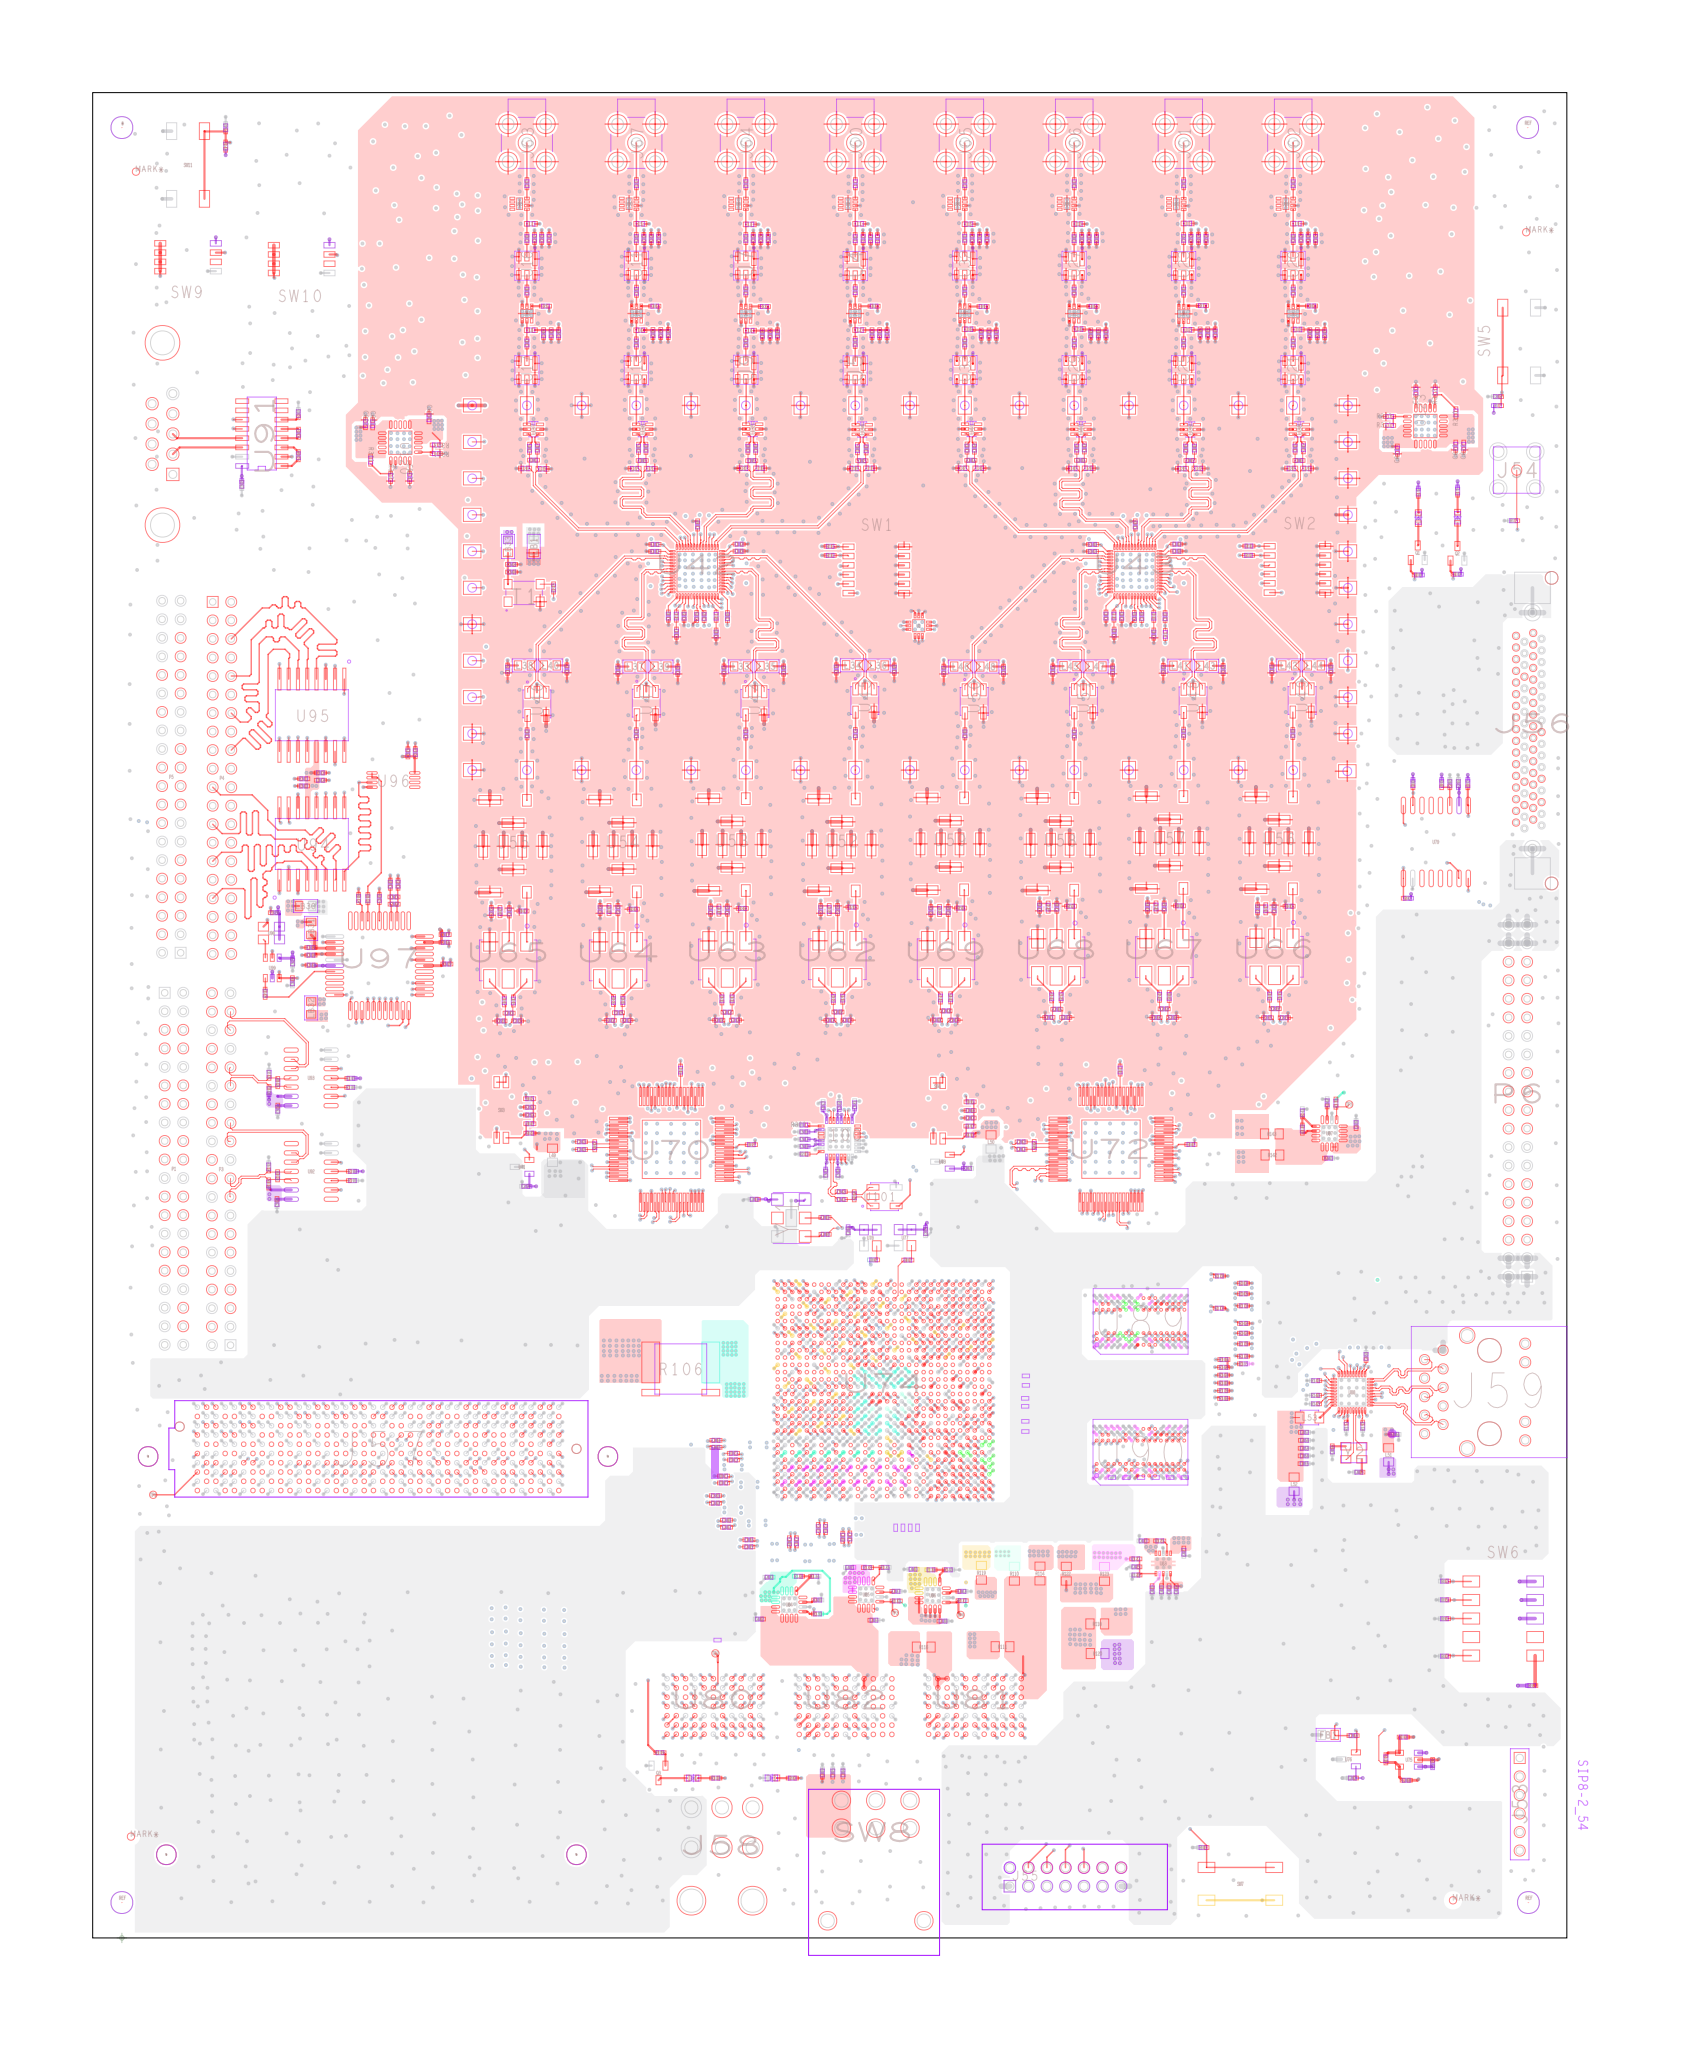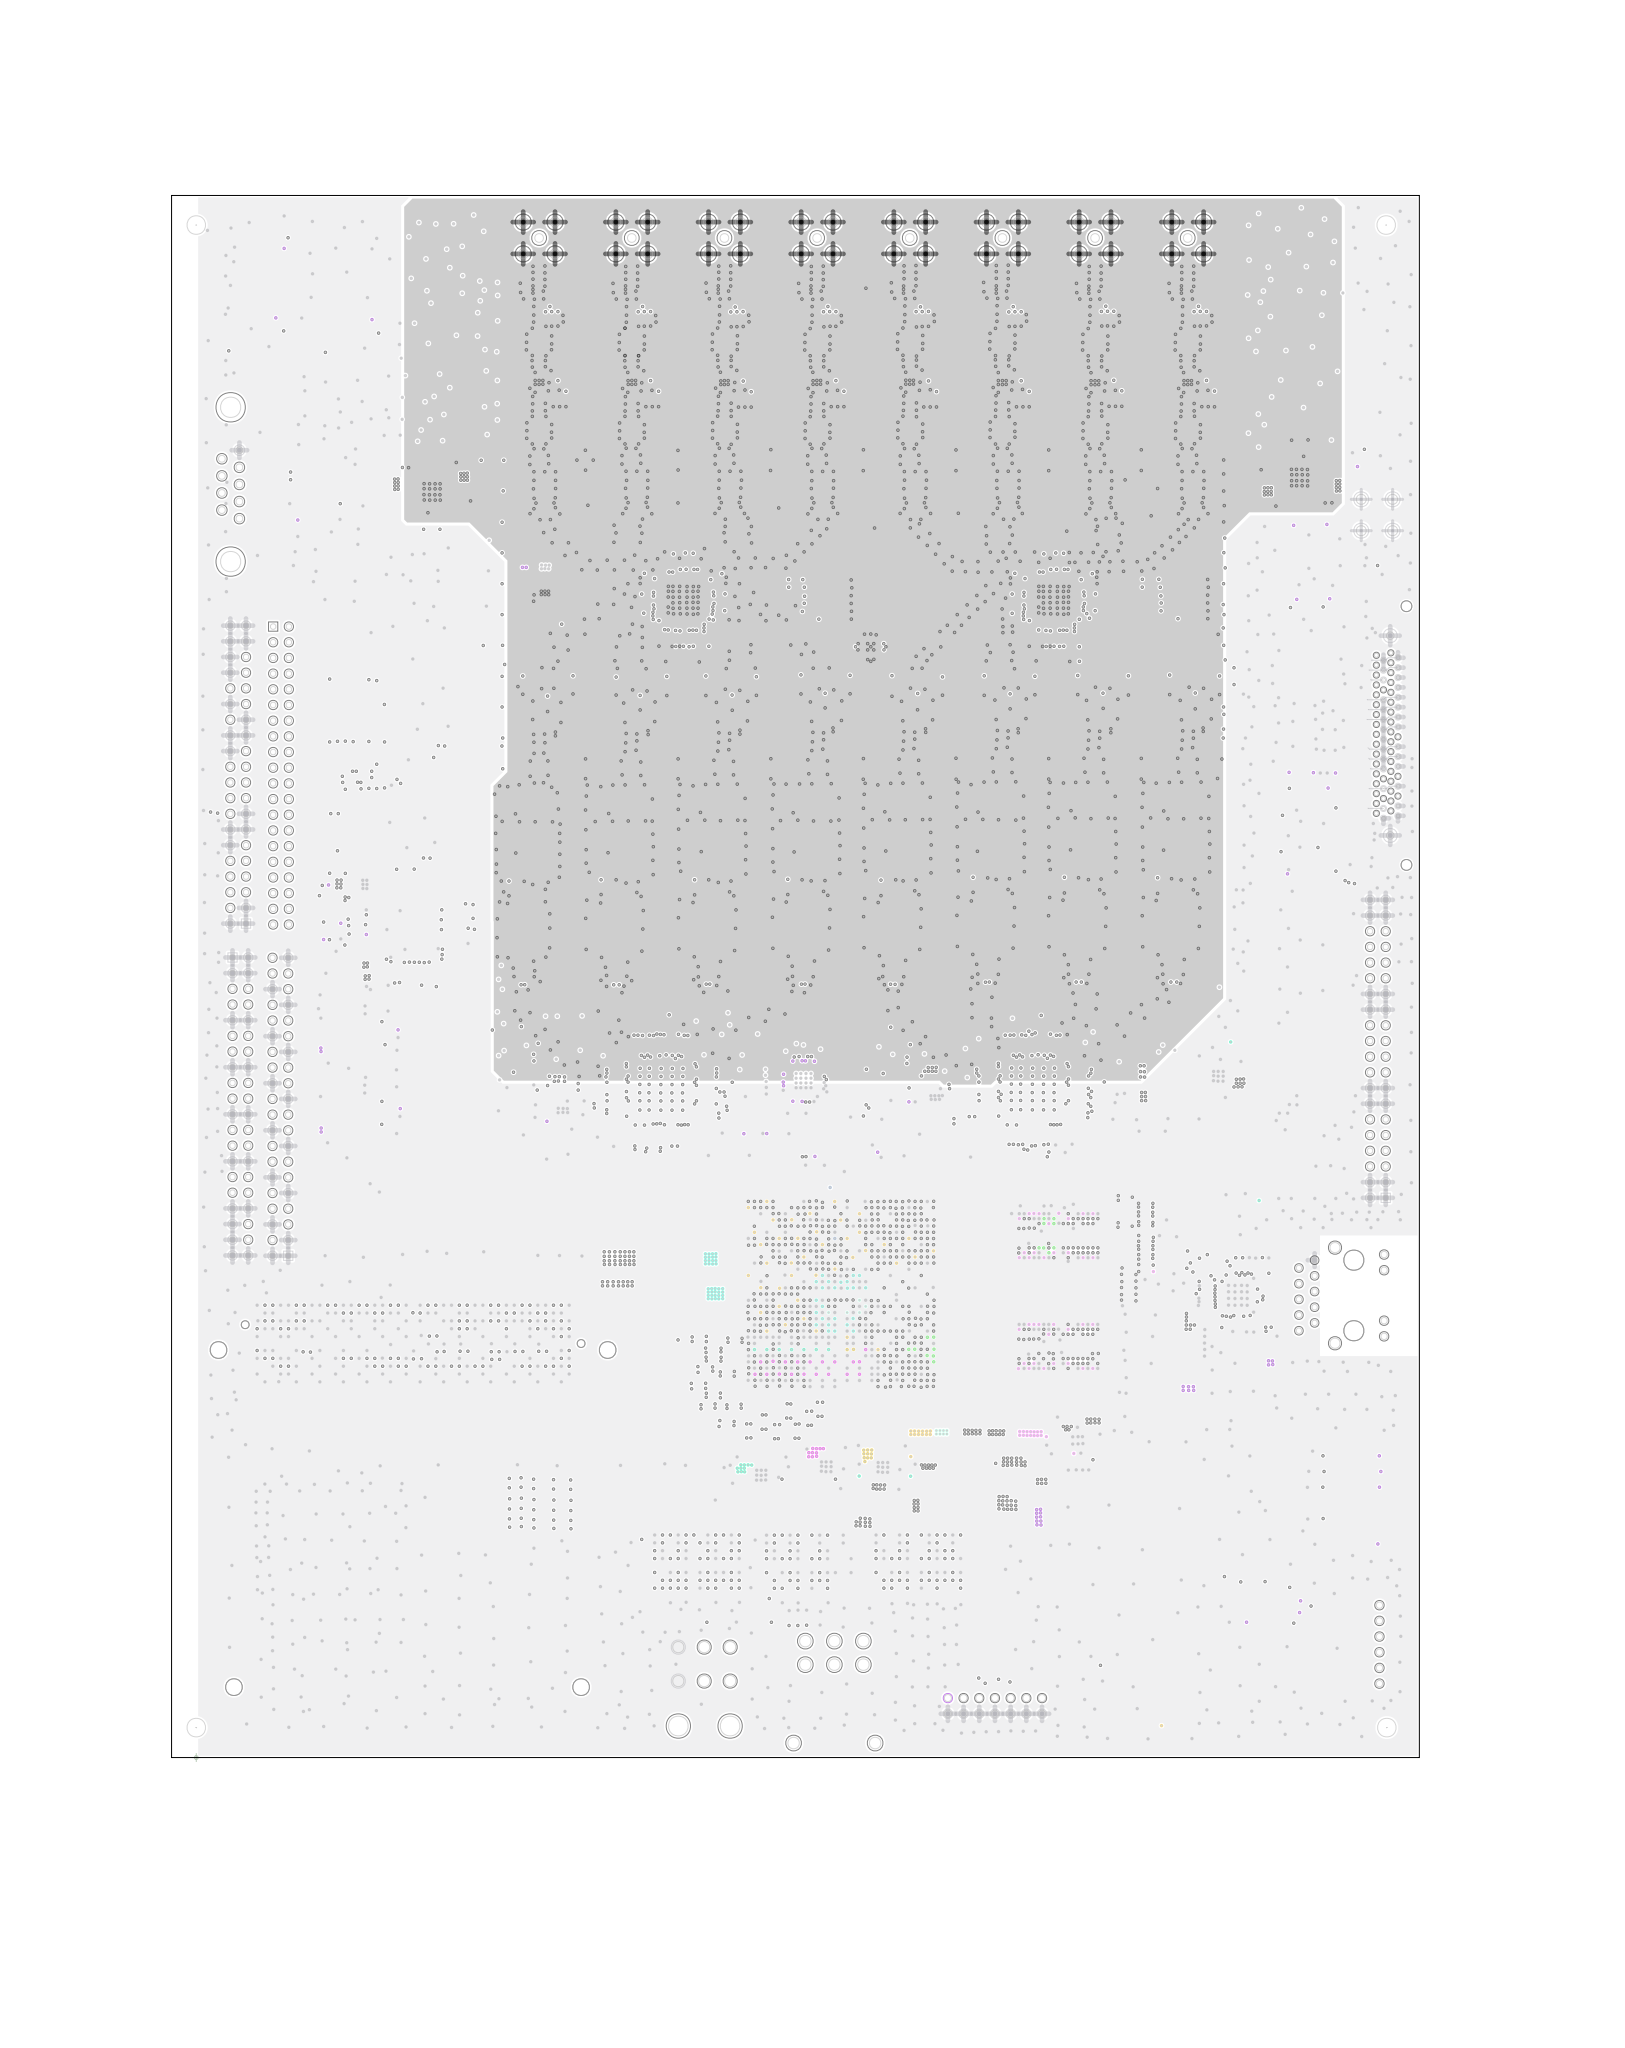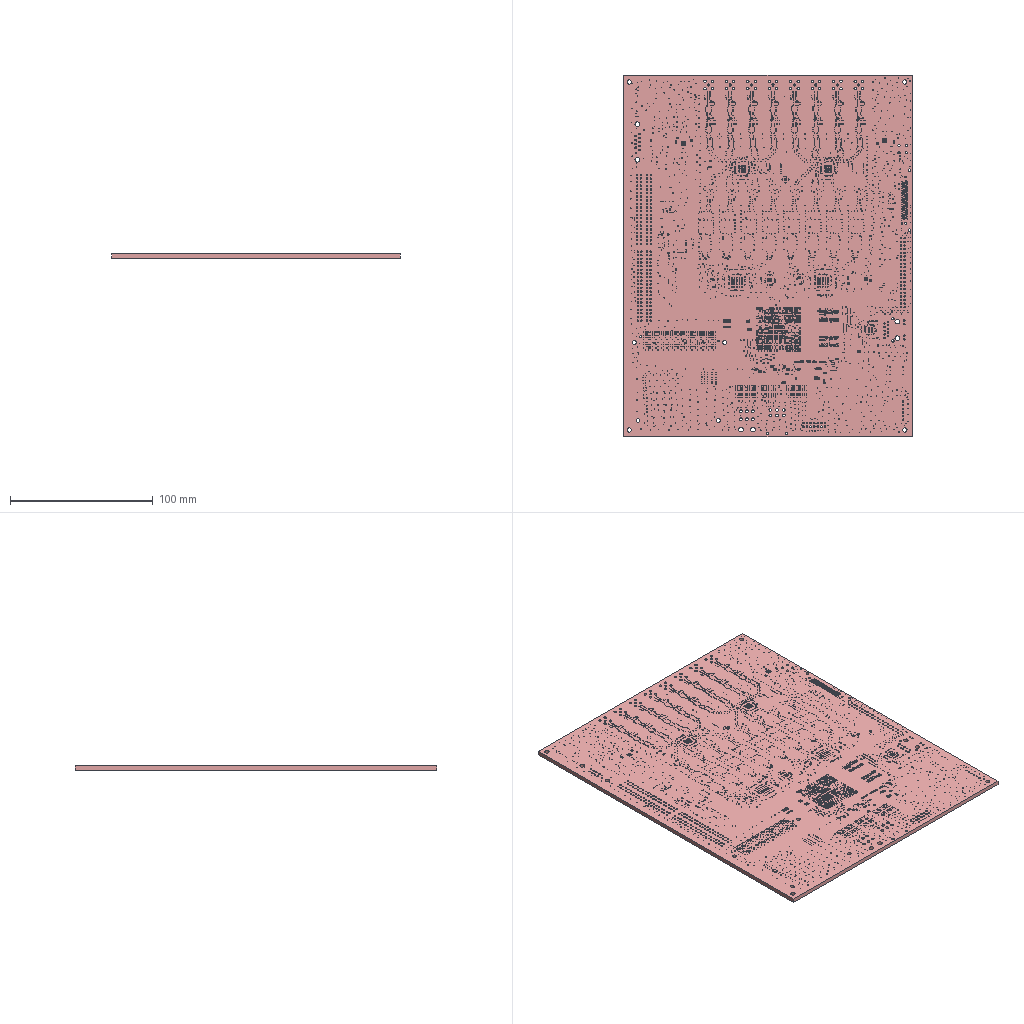Circuit board layout | Cadence Allegro | box 202 x 253 x 3 mm
Layer stack:
# Cadence Allegro layer stack of  (unit mm; from the constraint file cross-section; dielectric type: 0 not recorded (Allegro does not mark core vs prepreg), 3 surface material)
index,name,kind,layer,copper_thickness_mm,dielectric_type,dielectric_thickness_mm,dielectric_material,dielectric_constant
0,Top Surface,other,,,,,,
1,TOP,copper,TOP,0.0305,,,,
2,Dielectric1,dielectric,,,0,0.2032,FR-4,4.5
3,GND02,copper,GND02,0.0305,,,,
4,Dielectric2,dielectric,,,0,0.2032,FR-4,4.5
5,ART03,copper,ART03,0.0305,,,,
6,Dielectric3,dielectric,,,0,0.2032,FR-4,4.5
7,GND04,copper,GND04,0.0305,,,,
8,Dielectric4,dielectric,,,0,0.2032,FR-4,4.5
9,ART05,copper,ART05,0.0305,,,,
10,Dielectric5,dielectric,,,0,0.2032,FR-4,4.5
11,GND06,copper,GND06,0.0305,,,,
12,Dielectric6,dielectric,,,0,0.2032,FR-4,4.5
13,PWR07,copper,PWR07,0.0305,,,,
14,Dielectric7,dielectric,,,0,0.2032,FR-4,4.5
15,PWR08,copper,PWR08,0.0305,,,,
16,Dielectric8,dielectric,,,0,0.2032,FR-4,4.5
17,GND09,copper,GND09,0.0305,,,,
18,Dielectric9,dielectric,,,0,0.2032,FR-4,4.5
19,ART10,copper,ART10,0.0305,,,,
20,Dielectric10,dielectric,,,0,0.2032,FR-4,4.5
21,GND11,copper,GND11,0.0305,,,,
22,Dielectric11,dielectric,,,0,0.2032,FR-4,4.5
23,ART12,copper,ART12,0.0305,,,,
24,Dielectric12,dielectric,,,0,0.2032,FR-4,4.5
25,GND13,copper,GND13,0.0305,,,,
26,Dielectric13,dielectric,,,0,0.2032,FR-4,4.5
27,BOTTOM,copper,BOTTOM,0.0305,,,,
28,Bottom Surface,other,,,,,,
# drill layer pairs: low layer,high layer
drill_pair,TOP,BOTTOM
Part placement, first 520 of 1035 lines:
REFDES,COMP_VALUE,SYM_NAME,SYM_X,SYM_Y,SYM_ROTATE,SYM_MIRROR
C1,0.1uF,C0402,103.534,232.955,90.000,NO
C2,1000pF,C0402,101.578,232.98,90.000,NO
C3,10nF,C0402,102.594,232.955,90.000,NO
C4,0.1uF,C0402,104.851,219.939,90.000,NO
C5,1000pF,C0402,103.835,219.939,90.000,NO
C6,10nF,C0402,102.794,219.939,90.000,NO
C7,10nF,C0402,100.502,240.512,270.000,NO
C8,10nF,C0402,100.486,232.98,270.000,NO
C9,10nF,C0402,100.486,225.843,270.000,NO
C10,10nF,C0402,100.486,218.756,270.000,NO
C11,0.1uF,C0402,88.57,232.994,90.000,NO
C12,1000pF,C0402,86.512,232.994,90.000,NO
C13,10nF,C0402,87.554,232.994,90.000,NO
C14,0.1uF,C0402,89.84,219.913,90.000,NO
C15,1000pF,C0402,88.824,219.888,90.000,NO
C16,10nF,C0402,87.757,219.888,90.000,NO
C17,10nF,C0402,85.503,240.512,270.000,NO
C18,10nF,C0402,85.5,233.006,270.000,NO
C19,10nF,C0402,85.5,225.818,270.000,NO
C20,10nF,C0402,85.5,218.68,270.000,NO
C21,0.1uF,C0402,73.558,232.994,90.000,NO
C22,1000pF,C0402,71.526,232.994,90.000,NO
C23,10nF,C0402,72.542,232.994,90.000,NO
C24,0.1uF,C0402,72.771,219.964,90.000,NO
C25,1000pF,C0402,73.838,219.964,90.000,NO
C26,10nF,C0402,74.879,219.964,90.000,NO
C27,10nF,C0402,70.502,240.512,270.000,NO
C28,10nF,C0402,70.488,233.006,270.000,NO
C29,10nF,C0402,70.514,225.767,270.000,NO
C30,10nF,C0402,70.488,218.68,270.000,NO
C31,0.1uF,C0402,58.547,233.02,90.000,NO
C32,1000pF,C0402,56.54,233.02,90.000,NO
C33,10nF,C0402,57.531,233.02,90.000,NO
C34,0.1uF,C0402,57.785,219.939,90.000,NO
C35,1000pF,C0402,58.826,219.939,90.000,NO
C36,10nF,C0402,59.842,219.939,90.000,NO
C37,10nF,C0402,55.502,240.512,270.000,NO
C38,10nF,C0402,55.502,233.004,270.000,NO
C39,10nF,C0402,55.502,225.792,270.000,NO
C40,10nF,C0402,55.502,218.68,270.000,NO
C41,0.1uF,C0402,163.576,233.02,90.000,NO
C42,1000pF,C0402,161.569,233.02,90.000,NO
C43,10nF,C0402,162.56,233.045,90.000,NO
C44,0.1uF,C0402,164.821,219.939,90.000,NO
C45,1000pF,C0402,163.805,219.939,90.000,NO
C46,10nF,C0402,162.789,219.939,90.000,NO
C47,10nF,C0402,160.502,240.512,270.000,NO
C48,10nF,C0402,160.506,233.006,270.000,NO
C49,10nF,C0402,160.506,225.792,270.000,NO
C50,10nF,C0402,160.506,218.68,270.000,NO
C51,0.1uF,C0402,148.565,233.02,90.000,NO
C52,1000pF,C0402,146.482,233.02,90.000,NO
C53,10nF,C0402,147.523,233.02,90.000,NO
C54,0.1uF,C0402,149.809,220.04,90.000,NO
C55,1000pF,C0402,148.793,220.04,90.000,NO
C56,10nF,C0402,147.752,220.04,90.000,NO
C57,10nF,C0402,145.502,240.512,270.000,NO
C58,10nF,C0402,145.494,233.006,270.000,NO
C59,10nF,C0402,145.494,225.792,270.000,NO
C60,10nF,C0402,145.494,218.68,270.000,NO
C61,0.1uF,C0402,133.553,232.969,90.000,NO
C62,1000pF,C0402,131.521,232.994,90.000,NO
C63,10nF,C0402,132.537,232.969,90.000,NO
C64,0.1uF,C0402,134.849,219.913,90.000,NO
C65,1000pF,C0402,133.807,219.913,90.000,NO
C66,10nF,C0402,132.766,219.913,90.000,NO
C67,10nF,C0402,130.502,240.512,270.000,NO
C68,10nF,C0402,130.483,232.98,270.000,NO
C69,10nF,C0402,130.483,225.792,270.000,NO
C70,10nF,C0402,130.508,218.68,270.000,NO
C71,0.1uF,C0402,118.542,233.045,90.000,NO
C72,1000pF,C0402,116.51,233.02,90.000,NO
C73,10nF,C0402,117.526,233.02,90.000,NO
C74,0.1uF,C0402,119.812,219.888,90.000,NO
C75,1000pF,C0402,118.821,219.888,90.000,NO
C76,10nF,C0402,117.754,219.888,90.000,NO
C77,10nF,C0402,115.502,240.512,270.000,NO
C78,10nF,C0402,115.497,233.031,270.000,NO
C79,10nF,C0402,115.497,225.792,270.000,NO
C80,10nF,C0402,115.497,218.68,270.000,NO
C81,39pF,C0402,100.794,204.186,270.000,NO
C82,NC,C0402,101.404,202.535,180.000,NO
C83,39pF,C0402,101.988,204.161,270.000,NO
C84,39pF,C0402,85.783,204.237,270.000,NO
C85,NC,C0402,86.309,202.54,180.000,NO
C86,39pF,C0402,86.85,204.237,270.000,NO
C87,39pF,C0402,70.797,204.237,270.000,NO
C88,NC,C0402,71.305,202.56,180.000,NO
C89,39pF,C0402,71.813,204.237,270.000,NO
C90,39pF,C0402,55.861,204.237,270.000,NO
C91,NC,C0402,56.395,202.611,180.000,NO
C92,39pF,C0402,56.928,204.262,270.000,NO
C93,39pF,C0402,160.763,204.262,270.000,NO
C94,NC,C0402,161.297,202.56,180.000,NO
C95,39pF,C0402,161.906,204.313,270.000,NO
C96,39pF,C0402,145.777,204.262,270.000,NO
C97,NC,C0402,146.362,202.56,180.000,NO
C98,39pF,C0402,146.971,204.262,270.000,NO
C99,39pF,C0402,130.842,204.262,270.000,NO
C100,NC,C0402,131.369,202.59,180.000,NO
C101,39pF,C0402,131.883,204.288,270.000,NO
C102,39pF,C0402,115.805,204.262,270.000,NO
C103,NC,C0402,116.332,202.59,180.000,NO
C104,39pF,C0402,116.822,204.262,270.000,NO
C105,10nF,C0402,79.781,181.178,90.000,NO
C106,10nF,C0402,82.982,181.153,270.000,NO
C107,NC,C0402,75.997,178.892,270.000,NO
C108,NC,C0402,76.403,183.82,270.000,YES
C109,NC,C0402,81.432,178.765,270.000,NO
C110,NC,C0402,81.458,183.845,270.000,YES
C111,1uF,C0402,79.451,190.805,270.000,YES
C112,1uF,C0402,84.582,191.094,180.000,NO
C113,1uF,C0402,80.467,190.805,270.000,YES
C114,1uF,C0402,77.165,190.83,270.000,YES
C115,1uF,C0402,73.05,191.059,0.000,NO
C116,1uF,C0402,82.398,188.9,180.000,YES
C117,1uF,C0402,82.372,187.935,180.000,YES
C118,1uF,C0402,75.26,187.96,0.000,YES
C119,1uF,C0402,75.26,188.9,0.000,YES
C120,1uF,C0402,75.235,185.395,0.000,YES
C121,1uF,C0402,77.419,183.845,90.000,YES
C122,1uF,C0402,78.435,183.845,90.000,YES
C123,1uF,C0402,82.372,185.953,180.000,YES
C124,1uF,C0402,79.451,183.845,90.000,YES
C125,1uF,C0402,84.582,190.128,0.000,NO
C126,1uF,C0402,82.398,186.969,0.000,YES
C127,1uF,C0402,80.467,183.845,270.000,YES
C128,1uF,C0402,78.765,181.178,270.000,NO
C129,1uF,C0402,77.038,181.204,270.000,NO
C130,1uF,C0402,74.879,181.229,270.000,NO
C131,1uF,C0402,75.235,186.334,180.000,YES
C132,1uF,C0402,73.025,190.094,180.000,NO
C133,1uF,C0402,76.175,190.83,90.000,YES
C134,33nF,C0402,78.892,193.726,90.000,NO
C135,1uF,C0402,81.432,190.83,90.000,YES
C136,10nF,C0402,139.751,181.178,90.000,NO
C137,10nF,C0402,142.951,181.153,270.000,NO
C138,NC,C0402,135.966,178.892,270.000,NO
C139,NC,C0402,136.373,183.82,270.000,YES
C140,NC,C0402,141.402,178.765,270.000,NO
C141,NC,C0402,141.427,183.845,270.000,YES
C142,1uF,C0402,139.421,190.822,270.000,YES
C143,1uF,C0402,144.552,191.094,180.000,NO
C144,1uF,C0402,140.437,190.805,270.000,YES
C145,1uF,C0402,137.135,190.83,270.000,YES
C146,1uF,C0402,133.02,191.059,0.000,NO
C147,1uF,C0402,142.367,188.9,180.000,YES
C148,1uF,C0402,142.342,187.935,180.000,YES
C149,1uF,C0402,135.23,187.96,0.000,YES
C150,1uF,C0402,135.23,188.9,0.000,YES
C151,1uF,C0402,135.204,185.395,0.000,YES
C152,1uF,C0402,137.389,183.845,90.000,YES
C153,1uF,C0402,138.405,183.845,90.000,YES
C154,1uF,C0402,142.342,185.953,180.000,YES
C155,1uF,C0402,139.421,183.845,90.000,YES
C156,1uF,C0402,144.552,190.128,0.000,NO
C157,1uF,C0402,142.367,186.969,0.000,YES
C158,1uF,C0402,140.437,183.845,270.000,YES
C159,1uF,C0402,138.735,181.178,270.000,NO
C160,1uF,C0402,137.008,181.204,270.000,NO
C161,1uF,C0402,134.849,181.229,270.000,NO
C162,1uF,C0402,135.204,186.334,180.000,YES
C163,1uF,C0402,132.994,190.094,180.000,NO
C164,1uF,C0402,136.144,190.852,90.000,YES
C165,33nF,C0402,138.862,193.726,90.000,NO
C166,1uF,C0402,141.402,190.83,90.000,YES
C167,0.1uF,C0402,82.499,173.83,270.000,NO
C168,0.1uF,C0402,105.842,173.957,270.000,NO
C169,0.1uF,C0402,90.678,173.83,270.000,NO
C170,0.1uF,C0402,97.892,173.982,270.000,NO
C171,1nF,C0402,101.803,171.247,270.000,YES
C172,1nF,C0402,86.766,170.84,270.000,YES
C173,10nF,C0402,100.508,165.116,270.000,NO
C174,10nF,C0402,85.496,165.065,270.000,NO
C175,0.1uF,C0402,52.857,173.957,270.000,NO
C176,0.1uF,C0402,76.175,173.804,270.000,NO
C177,0.1uF,C0402,60.985,173.982,270.000,NO
C178,0.1uF,C0402,67.97,173.83,270.000,NO
C179,1nF,C0402,71.857,170.891,270.000,YES
C180,1nF,C0402,56.871,170.79,270.000,YES
C181,10nF,C0402,70.485,165.091,270.000,NO
C182,10nF,C0402,55.524,165.091,270.000,NO
C183,0.1uF,C0402,150.901,173.906,270.000,NO
C184,0.1uF,C0402,157.582,173.957,270.000,NO
C185,0.1uF,C0402,142.697,173.906,270.000,NO
C186,0.1uF,C0402,165.659,173.957,270.000,NO
C187,1nF,C0402,161.722,171.247,270.000,YES
C188,1nF,C0402,146.812,171.196,270.000,YES
C189,10nF,C0402,160.452,165.141,270.000,NO
C190,10nF,C0402,145.491,165.167,270.000,NO
C191,0.1uF,C0402,127.559,173.83,270.000,NO
C192,0.1uF,C0402,112.624,173.804,270.000,NO
C193,0.1uF,C0402,135.763,173.83,270.000,NO
C194,0.1uF,C0402,120.802,173.804,270.000,NO
C195,1nF,C0402,131.75,171.12,270.000,YES
C196,1nF,C0402,116.764,171.12,270.000,YES
C197,10nF,C0402,130.505,165.065,270.000,NO
C198,10nF,C0402,115.519,165.091,270.000,NO
C207,5pF,C0402,99.365,125.832,180.000,NO
C208,5pF,C0402,98.12,126.949,0.000,NO
C209,0.1uF,C0402,98.069,140.995,270.000,NO
C210,0.1uF,C0402,95.758,140.995,90.000,NO
C211,5pF,C0402,97.028,125.822,0.000,NO
C212,5pF,C0402,84.074,125.832,180.000,NO
C213,5pF,C0402,82.931,126.924,0.000,NO
C214,0.1uF,C0402,82.956,140.919,270.000,NO
C215,0.1uF,C0402,80.67,140.919,90.000,NO
C216,5pF,C0402,81.788,125.822,0.000,NO
C217,5pF,C0402,69.19,125.806,180.000,NO
C218,5pF,C0402,68.047,126.848,0.000,NO
C219,0.1uF,C0402,67.97,140.986,270.000,NO
C220,0.1uF,C0402,65.532,140.986,90.000,NO
C221,5pF,C0402,66.929,125.806,0.000,NO
C222,5pF,C0402,54.204,125.73,180.000,NO
C223,5pF,C0402,53.061,126.797,0.000,NO
C224,0.1uF,C0402,53.086,140.681,270.000,NO
C225,0.1uF,C0402,50.622,140.716,90.000,NO
C226,5pF,C0402,51.943,125.721,0.000,NO
C227,5pF,C0402,159.283,126.162,180.000,NO
C228,5pF,C0402,158.039,127.406,0.000,NO
C229,0.1uF,C0402,157.886,141.097,270.000,NO
C230,0.1uF,C0402,155.626,141.097,90.000,NO
C231,5pF,C0402,156.972,126.162,0.000,NO
C232,5pF,C0402,143.993,126.213,180.000,NO
C233,5pF,C0402,142.824,127.381,0.000,NO
C234,0.1uF,C0402,142.824,141.351,270.000,NO
C235,0.1uF,C0402,140.538,141.351,90.000,NO
C236,5pF,C0402,141.707,126.187,0.000,NO
C237,5pF,C0402,129.337,126.213,180.000,NO
C238,5pF,C0402,128.118,127.33,0.000,NO
C239,0.1uF,C0402,128.118,141.326,270.000,NO
C240,0.1uF,C0402,125.755,141.326,90.000,NO
C241,5pF,C0402,127.025,126.213,0.000,NO
C242,5pF,C0402,114.021,125.832,180.000,NO
C243,5pF,C0402,112.928,127.102,0.000,NO
C244,0.1uF,C0402,113.233,140.868,270.000,NO
C245,0.1uF,C0402,110.846,140.843,90.000,NO
C246,5pF,C0402,111.633,125.848,0.000,NO
C247,0.1uF,C0402,62.966,109.16,180.000,NO
C248,0.1uF,C0402,62.966,108.093,180.000,NO
C249,10uF,C0402,75.032,115.621,270.000,YES
C250,10uF,C0402,55.347,103.048,0.000,NO
C251,1.0uF,C0402,55.88,113.894,180.000,NO
C252,0.1uF,C0402,55.88,112.827,0.000,NO
C253,0.1uF,C0402,67.869,106.35,0.000,YES
C254,0.1uF,C0402,82.779,105.867,180.000,YES
C255,0.1uF,C0402,67.843,107.391,0.000,YES
C256,0.1uF,C0402,78.054,115.621,270.000,YES
C257,0.1uF,C0402,82.956,110.388,180.000,YES
C258,0.1uF,C0402,73.533,115.621,270.000,YES
C259,0.1uF,C0402,67.843,110.338,0.000,YES
C260,0.1uF,C0402,72.06,115.57,270.000,YES
C261,0.1uF,C0402,67.843,109.347,0.000,YES
C262,0.1uF,C0402,123.231,109.144,180.000,NO
C263,0.1uF,C0402,123.199,108.128,180.000,NO
C264,10uF,C0402,135.28,115.621,270.000,YES
C265,10uF,C0402,115.875,105.512,180.000,NO
C266,1.0uF,C0402,116.23,113.436,180.000,NO
C267,0.1uF,C0402,116.23,112.42,0.000,NO
C268,0.1uF,C0402,128.092,106.375,0.000,YES
C269,0.1uF,C0402,143.002,105.893,180.000,YES
C270,0.1uF,C0402,128.067,109.372,0.000,YES
C271,0.1uF,C0402,128.067,107.417,0.000,YES
C272,0.1uF,C0402,138.278,115.646,270.000,YES
C273,0.1uF,C0402,132.283,115.595,270.000,YES
C274,0.1uF,C0402,143.213,110.414,180.000,YES
C275,0.1uF,C0402,133.756,115.646,270.000,YES
C276,0.1uF,C0402,128.067,110.363,0.000,YES
C277,0.1uF/25V/X2R,C0402_BGA,103.327,73.584,180.000,YES
C278,0.1uF/25V/X2R,C0402_BGA,104.851,73.05,90.000,YES
C279,10uF,C0402,179.603,23.901,270.000,NO
C280,10uF,C0402,175.997,21.615,180.000,NO
C281,47uF/10V/X5R,C0402_BGA,104.877,69.063,90.000,YES
C282,10uF,C0402,168.605,21.92,0.000,NO
C283,10uF/10V,C0402,188.493,211.328,0.000,NO
C284,10uF,C0402,168.707,27.737,0.000,NO
C285,0.1uF,C0402,110.134,96.85,90.000,NO
C286,0.1uF,C0402,99.517,96.952,90.000,NO
C287,100uF/6.3V/X5R,C0402_BGA,100.355,83.566,180.000,YES
C288,100uF/6.3V/X5R,C0402_BGA,105.893,85.065,90.000,YES
C289,0.1uF,C0402,96.342,98.781,180.000,NO
C290,0.1uF,C0402,96.368,96.469,180.000,NO
C291,0.1uF,C0402,86.639,101.27,0.000,NO
C292,0.1uF,C0402,183.134,158.267,270.000,NO
C293,0.1uF,C0402,181.966,158.267,270.000,NO
C294,0.1uF/25V/X7R,C0402_BGA,114.351,73.609,0.000,YES
C295,0.1uF/25V/X7R,C0402_BGA,114.351,72.568,0.000,YES
C296,0.1uF/25V/X7R,C0402_BGA,116.357,76.581,180.000,YES
C297,0.1uF/25V/X7R,C0402_BGA,111.887,71.095,90.000,YES
C298,100uF/6.3V/X5R,C0402_BGA,114.351,69.571,0.000,YES
C299,100uF/6.3V/X5R,C0402_BGA,113.386,77.572,180.000,YES
C300,0.1uF/25V/X7R,C0402_BGA,113.386,66.599,0.000,YES
C301,0.1uF/25V/X7R,C0402_BGA,115.341,67.589,0.000,YES
C302,100uF/6.3V/X5R,C0402_BGA,112.852,61.112,270.000,YES
C303,100uF/6.3V/X5R,C0402_BGA,111.379,88.57,0.000,YES
C304,0.1uF,C0402,81.407,68.224,0.000,NO
C305,0.1uF,C0402,81.407,67.259,0.000,NO
C306,0.1uF,C0402,82.448,63.322,0.000,NO
C307,0.1uF,C0402,85.979,62.611,180.000,YES
C308,0.1uF,C0402,85.954,61.62,180.000,YES
C309,0.1uF,C0402,91.465,54.305,90.000,NO
C310,0.1uF,C0402,82.448,62.382,0.000,NO
C311,0.1uF,C0402,92.431,54.305,90.000,NO
C312,0.1uF,C0402,83.795,65.532,0.000,NO
C313,0.1uF,C0402,87.224,67.056,180.000,YES
C314,0.1uF,C0402,83.795,66.446,0.000,NO
C315,0.1uF,C0402,87.224,68.021,180.000,YES
C316,0.1uF,C0402,83.769,64.999,180.000,YES
C317,0.1uF,C0402,95.428,56.134,90.000,NO
C318,0.1uF,C0402,83.769,64.084,180.000,YES
C319,0.1uF,C0402,96.418,56.134,90.000,NO
C320,0.1uF,C0402,87.071,57.302,180.000,YES
C321,0.1uF,C0402,101.473,56.413,270.000,YES
C322,0.1uF,C0402,87.071,56.388,180.000,YES
C323,0.1uF,C0402,100.508,56.413,270.000,YES
C324,0.1uF,C0402,96.774,52.857,90.000,YES
C325,0.1uF,C0402,97.714,52.857,90.000,YES
C326,0.1uF,C0402,98.781,54.94,270.000,NO
C327,0.1uF,C0402,99.746,54.966,270.000,NO
C328,0.1uF,C0402,93.497,52.781,90.000,YES
C329,0.1uF,C0402,94.437,52.781,90.000,YES
C330,0.1uF,C0402,88.951,52.908,90.000,YES
C331,0.1uF,C0402,89.941,52.908,90.000,YES
C332,0.1uF,C0402,81.331,60.63,0.000,NO
C333,0.1uF,C0402,81.331,59.614,0.000,NO
C334,0.1uF,C0402,85.928,54.585,180.000,NO
C335,0.1uF,C0402,85.903,53.619,180.000,NO
C336,0.1uF,C0402,82.855,57.277,0.000,NO
C337,0.1uF,C0402,82.855,56.312,0.000,NO
C338,0.1uF,C0402,83.718,59.131,0.000,YES
C339,0.1uF,C0402,83.718,58.166,0.000,YES
C340,100uF/6.3V/X5R,C0402_BGA,116.357,83.566,0.000,YES
C341,100uF/6.3V/X5R,C0402_BGA,106.883,82.042,90.000,YES
C342,100uF/6.3V/X5R,C0402_BGA,94.869,83.083,270.000,YES
C343,100uF/6.3V/X5R,C0402_BGA,93.853,72.06,270.000,YES
C344,4.7uF/6.3V/X5R,C0402_BGA,102.362,74.803,180.000,YES
C345,4.7uF/6.3V/X5R,C0402_BGA,102.358,76.574,180.000,YES
C346,4.7uF/6.3V/X5R,C0402_BGA,104.419,75.667,180.000,YES
C347,4.7uF/6.3V/X5R,C0402_BGA,104.419,76.556,180.000,YES
C348,4.7uF/6.3V/X5R,C0402_BGA,108.407,76.556,0.000,YES
C349,4.7uF/6.3V/X5R,C0402_BGA,100.355,74.803,180.000,YES
C350,4.7uF/6.3V/X5R,C0402_BGA,100.358,76.574,180.000,YES
C351,4.7uF/6.3V/X5R,C0402_BGA,100.355,75.641,180.000,YES
C352,4.7uF/6.3V/X5R,C0402_BGA,108.407,75.616,0.000,YES
C353,330uF/10V/TANT,C0402_BGA,102.362,75.667,0.000,YES
C354,330uF/10V/TANT,C0402_BGA,102.387,69.596,0.000,YES
C355,330uF/10V/TANT,C0402_BGA,107.366,77.572,180.000,YES
C356,330uF/10V/TANT,C0402_BGA,101.346,71.603,180.000,YES
C357,330uF/10V/TANT,C0402_BGA,106.858,72.085,270.000,YES
C358,330uF/10V/TANT,C0402_BGA,101.371,77.572,0.000,YES
C359,47uF/10V/X5R,C0402_BGA,102.362,72.517,0.000,YES
C360,47uF/10V/X5R,C0402_BGA,107.899,72.06,270.000,YES
C361,47uF/10V/X5R,C0402_BGA,108.204,74.574,0.000,YES
C362,47uF/10V/X5R,C0402_BGA,107.899,70.053,90.000,YES
C363,0.022uF/10V/X5R,C0402_BGA,99.873,61.062,270.000,YES
C364,0.022uF/10V/X5R,C0402_BGA,97.892,61.087,270.000,YES
C365,0.022uF/10V/X5R,C0402_BGA,95.91,61.062,270.000,YES
C366,0.022uF/10V/X5R,C0402_BGA,102.87,64.084,90.000,YES
C367,0.022uF/10V/X5R,C0402_BGA,93.929,66.091,90.000,YES
C368,0.022uF/10V/X5R,C0402_BGA,100.813,66.091,90.000,YES
C369,0.022uF/10V/X5R,C0402_BGA,91.948,65.1,270.000,YES
C370,0.022uF/10V/X5R,C0402_BGA,101.879,66.091,90.000,YES
C371,0.022uF/10V/X5R,C0402_BGA,105.893,65.024,270.000,YES
C372,0.022uF/10V/X5R,C0402_BGA,104.927,65.049,270.000,YES
C373,0.022uF/10V/X5R,C0402_BGA,104.927,67.081,90.000,YES
C374,0.022uF/10V/X5R,C0402_BGA,105.893,67.031,90.000,YES
C375,0.47uF/10V/X5R,C0402_BGA,93.929,61.062,270.000,YES
C376,0.47uF/10V/X5R,C0402_BGA,101.93,61.036,270.000,YES
C377,0.47uF/10V/X5R,C0402_BGA,107.874,61.087,270.000,YES
C378,0.47uF/10V/X5R,C0402_BGA,107.874,63.094,270.000,YES
C379,0.47uF/10V/X5R,C0402_BGA,89.865,66.116,90.000,YES
C380,0.47uF/10V/X5R,C0402_BGA,95.91,66.091,90.000,YES
C381,0.47uF/10V/X5R,C0402_BGA,96.85,66.091,90.000,YES
C382,0.47uF/10V/X5R,C0402_BGA,98.831,65.101,270.000,YES
C383,1uF/25V/X5R,C0402_BGA,91.872,61.062,270.000,YES
C384,1uF/25V/X5R,C0402_BGA,89.916,61.138,270.000,YES
C385,4.7uF/6.3V/X5R,C0402_BGA,105.842,61.062,270.000,YES
C386,4.7uF/6.3V/X5R,C0402_BGA,108.839,65.024,270.000,YES
C387,1uF/25V/X5R,C0402_BGA,92.888,65.1,270.000,YES
C388,1uF/25V/X5R,C0402_BGA,97.917,65.1,270.000,YES
C389,4.7uF/6.3V/X5R,C0402_BGA,91.008,66.116,90.000,YES
C390,4.7uF/6.3V/X5R,C0402_BGA,94.996,66.091,90.000,YES
C391,47uF,C0402,78.664,35.433,0.000,YES
C392,47uF,C0402,74.854,35.484,0.000,YES
C393,47uF,C0402,83.439,35.433,0.000,YES
C394,47uF,C0402,98.806,22.631,270.000,NO
C395,10uF,C0402,97.409,22.622,270.000,NO
C396,10uF,C0402,87.224,31.648,0.000,YES
C397,47uF,C0402,87.249,35.458,0.000,YES
C398,100uF/16V,C0402,83.439,31.623,180.000,YES
C399,10uF,C0402,95.986,22.622,270.000,NO
C400,0.1uF,C0402,79.858,29.464,90.000,YES
C401,10uF,C0402,78.613,31.648,0.000,YES
C402,4.7uF,C0402,77.572,29.337,180.000,YES
C403,10uF,C0402,74.778,31.674,0.000,YES
C404,10uF,C0402,123.038,31.674,0.000,YES
C405,10uF,C0402,119.202,31.648,0.000,YES
C406,47uF,C0402,123.012,35.433,0.000,YES
C407,0.1uF,C0402,124.384,29.388,90.000,YES
C408,47uF,C0402,119.202,35.458,0.000,YES
C409,0.1uF,C0402,120.574,29.388,90.000,YES
C410,47uF,C0402,114.529,35.458,0.000,YES
C411,10uF,C0402,114.529,31.648,0.000,YES
C412,0.1uF,C0402,115.748,29.388,90.000,YES
C413,47uF,C0402,110.82,35.484,0.000,YES
C414,10uF,C0402,110.719,31.674,0.000,YES
C415,0.1uF,C0402,111.963,29.388,90.000,YES
C416,10uF,C0402,101.524,31.623,0.000,YES
C417,47uF,C0402,101.498,35.433,0.000,YES
C418,0.1uF,C0402,102.616,29.286,0.000,YES
C419,10uF,C0402,96.774,31.648,0.000,YES
C420,47uF,C0402,96.825,35.382,0.000,YES
C421,0.1uF,C0402,98.146,29.489,90.000,YES
C422,47uF,C0402,92.939,35.408,0.000,YES
C423,10uF,C0402,92.913,31.623,0.000,YES
C424,0.1uF,C0402,94.234,29.388,90.000,YES
C425,1nF,C0402,138.938,50.876,0.000,NO
C426,10uF,C0402,141.173,47.727,270.000,NO
C427,0.1uF,C0402,145.517,52.883,90.000,NO
C428,10uF,C0402,142.453,47.726,270.000,NO
C429,10uF,C0402,143.494,47.726,270.000,NO
C430,10uF,C0402,144.475,47.727,270.000,NO
C431,1uF,C0402,139.929,54.432,0.000,NO
C432,4.7uF/10V,C0402,87.351,43.713,0.000,NO
C433,4.7uF/10V,C0402,88.671,49.454,0.000,NO
C434,4.7uF/10V,C0402,103.057,43.561,180.000,NO
C435,4.7uF/10V,C0402,99.73,50.8,0.000,NO
C436,10nF,C0402,95.352,46.33,0.000,NO
C437,10nF,C0402,106.08,47.523,0.000,NO
C438,4.7uF/10V,C0402,112.522,43.434,180.000,NO
C439,4.7uF/10V,C0402,169.123,111.531,270.000,NO
C440,4.7uF/10V,C0402,108.407,50.546,0.000,NO
C441,4.7uF/10V,C0402,165.363,106.908,180.000,NO
C442,10nF,C0402,165.16,114.503,90.000,NO
C443,10nF,C0402,115.113,47.514,0.000,NO
C444,4.7uF/6.3V,C0402,174.447,69.037,0.000,NO
C445,0.1uF/6.3V,C0402,171.501,79.731,270.000,YES
C446,0.1uF/6.3V,C0402,171.196,70.155,90.000,YES
C447,4.7uF/6.3V,C0402,171.171,76.454,270.000,YES
C448,0.1uF/6.3V,C0402,171.171,73.279,90.000,YES
C449,0.1uF/6.3V,C0402,170.028,70.155,90.000,YES
C450,0.1uF/6.3V,C0402,173.634,79.731,270.000,YES
C451,100nF/6.3V,C0402,163.551,73.838,0.000,YES
C452,0.1uF/6.3V,C0402,163.525,72.923,0.000,YES
C453,4.7uF/6.3V,C0402,162.027,67.132,0.000,NO
C454,1uF/6.3V,C0402,162.027,66.091,0.000,NO
C455,100nF/6.3V,C0402,162.001,65.024,0.000,NO
C456,4.7uF/6.3V,C0402,162.052,68.224,0.000,NO
C457,0.1uF/6.3V,C0402,162.052,69.317,0.000,NO
C458,100nF/6.3V,C0402,170.485,79.731,90.000,NO
C459,18pF/6.3V,C0402,165.862,66.904,270.000,NO
C460,18pF/6.3V,C0402,169.494,63.856,180.000,NO
C461,0.1uF/10V,C0402,178.003,64.719,180.000,YES
C463,0.1uF,C0402,134.061,82.947,90.000,YES
C464,0.1uF,C0402,143.434,80.305,180.000,YES
C465,0.1uF,C0402,140.538,87.824,90.000,YES
C466,0.1uF,C0402,134.544,88.764,180.000,YES
C467,0.1uF,C0402,145.694,80.356,0.000,YES
C468,0.1uF,C0402,138.912,88.738,180.000,YES
C469,0.1uF,C0402,136.728,88.738,0.000,YES
C470,0.1uF,C0402,139.522,82.21,90.000,YES
C471,0.1uF,C0402,135.356,80.356,0.000,YES
C472,0.1uF,C0402,137.49,85.893,180.000,YES
C473,0.1uF,C0402,145.847,88.84,0.000,YES
C474,0.1uF,C0402,132.588,87.595,90.000,YES
C475,0.1uF,C0402,133.197,80.356,0.000,YES
C476,0.1uF,C0402,141.783,80.559,270.000,YES
C477,0.1uF,C0402,143.662,88.84,0.000,YES
C478,0.1uF,C0402,137.541,80.356,0.000,YES
C479,10uF,C0402,145.694,79.442,0.000,YES
C480,10uF,C0402,134.518,89.703,180.000,YES
C481,0.1uF,C0402,139.674,80.356,0.000,YES
C482,0.1uF,C0402,142.773,86.122,270.000,YES
C483,0.1uF,C0402,140.462,69.917,90.000,YES
C484,0.1uF,C0402,139.446,64.43,90.000,YES
C485,0.1uF,C0402,145.72,62.398,0.000,YES
C486,0.1uF,C0402,137.642,62.424,0.000,YES
C487,0.1uF,C0402,135.483,62.424,0.000,YES
C488,0.1uF,C0402,133.401,62.424,0.000,YES
C489,0.1uF,C0402,137.719,67.961,180.000,YES
C490,0.1uF,C0402,136.55,70.755,0.000,YES
C491,0.1uF,C0402,134.442,70.755,180.000,YES
C492,0.1uF,C0402,134.112,64.964,90.000,YES
C493,0.1uF,C0402,132.639,69.714,90.000,YES
C494,0.1uF,C0402,145.847,70.78,0.000,YES
C495,0.1uF,C0402,143.662,70.78,0.000,YES
C496,0.1uF,C0402,138.735,70.78,180.000,YES
C497,0.1uF,C0402,143.23,62.449,180.000,YES
C498,0.1uF,C0402,134.442,71.72,180.000,YES
C499,10uF,C0402,141.706,62.678,270.000,YES
C500,10uF,C0402,145.72,61.484,0.000,YES
C501,0.1uF,C0402,139.827,62.424,0.000,YES
C502,0.1uF,C0402,142.748,68.139,270.000,YES
C503,0.1uF,C0402,16.434,199.288,270.000,NO
C504,0.1uF,C0402,23.266,201.879,270.000,YES
C505,0.1uF,C0402,24.181,208.991,270.000,NO
C506,0.1uF,C0402,24.181,203.225,90.000,NO
C507,0.1uF,C0402,24.206,206.299,90.000,NO
C508,0.1uF,C0402,21.361,113.614,270.000,NO
C509,0.1uF,C0402,21.26,100.813,270.000,NO
C510,10uF,C0402,24.892,157.937,0.000,NO
C511,0.1uF,C0402,24.917,158.928,0.000,NO
C512,10uF,C0402,27.203,159.741,180.000,NO
C513,0.1uF,C0402,27.203,158.725,180.000,NO
C514,0.1uF,C0402,40.208,162.509,270.000,NO
C515,10uF,C0402,39.192,162.484,270.000,NO
C516,0.1uF,C0402,25.908,134.747,0.000,NO
C517,10uF/16V,C0402,44.298,137.566,0.000,NO
C518,0.1uF,C0402,44.298,136.5,180.000,NO
C519,0.1uF,C0402,44.526,133.528,180.000,NO
C520,0.1uF,C0402,36.779,144.475,90.000,NO
C521,10uF/16V,C0402,37.287,142.723,0.000,NO
C522,0.1uF,C0402,37.313,141.732,180.000,NO
C523,0.1uF,C0402,37.846,144.475,90.000,NO
C524,0.1uF,C0402,25.933,133.375,0.000,NO
C525,0.1uF,C0402,25.908,135.788,0.000,NO
C526,0.1uF,C0402,35.281,142.519,270.000,NO
C527,0.1uF,C0402,23.393,133.807,90.000,NO
C528,0.1uF,C0402,23.368,131.089,90.000,NO
Pad and via stacks, first 106 of 119 lines:
# Allegro (Cadence) via spans and padstacks; design units: ("millimeters" 4 10000)
# via spans: padstack,start_layer,end_layer,net_example,count
VIA8-F,ETCH/TOP,ETCH/BOTTOM,GND,5517
# Allegro padstack definitions: name,start_layer,end_layer,drill,plating,holeType,type
SMD_C197P0S40,"ETCH/TOP","ETCH/TOP",0.0,"PLATED","none","smd"
BALL25,"ETCH/TOP","ETCH/TOP",0.0,"NON_PLATED","none","smd"
BALL16M2,"ETCH/TOP","ETCH/TOP",0.0,"NON_PLATED","none","smd"
SMD_C250P0S40,"ETCH/TOP","ETCH/TOP",0.0,"PLATED","none","smd"
SMD10_40,"ETCH/TOP","ETCH/TOP",0.0,"NON_PLATED","none","smd"
SMD40_10,"ETCH/TOP","ETCH/TOP",0.0,"NON_PLATED","none","smd"
SMD283_283NP,"ETCH/TOP","ETCH/TOP",0.0,"NON_PLATED","none","smd"
SMD5_55-1,"ETCH/TOP","ETCH/TOP",0.0,"NON_PLATED","none","smd"
SMD0_75X0_2-1,"ETCH/TOP","ETCH/TOP",0.0,"NON_PLATED","none","smd"
R80_30,"ETCH/TOP","ETCH/TOP",0.0,"PLATED","none","smd"
R560_560,"ETCH/TOP","ETCH/TOP",0.0,"PLATED","none","smd"
SMD_O193X984P0S20,"ETCH/TOP","ETCH/TOP",0.0,"PLATED","none","smd"
SMD_O984X193P0S20,"ETCH/TOP","ETCH/TOP",0.0,"PLATED","none","smd"
SMD_O79X315P0S20,"ETCH/TOP","ETCH/TOP",0.0,"PLATED","none","smd"
SMD_S1496P0S20,"ETCH/TOP","ETCH/TOP",0.0,"PLATED","none","smd"
SMD_R315X118P0S20,"ETCH/TOP","ETCH/TOP",0.0,"PLATED","none","smd"
SMD_R118X315P0S20,"ETCH/TOP","ETCH/TOP",0.0,"PLATED","none","smd"
SMD_S1221P0S20,"ETCH/TOP","ETCH/TOP",0.0,"PLATED","none","smd"
SMD_O447X143P0S20,"ETCH/TOP","ETCH/TOP",0.0,"PLATED","none","smd"
SMD_O143X447P0S20,"ETCH/TOP","ETCH/TOP",0.0,"PLATED","none","smd"
SMD_S827P0S20,"ETCH/TOP","ETCH/TOP",0.0,"PLATED","none","smd"
SMD25_70,"ETCH/TOP","ETCH/TOP",0.0,"NON_PLATED","none","smd"
SMD_O236X906P0S20,"ETCH/TOP","ETCH/TOP",0.0,"PLATED","none","smd"
SMD_O234X775P0S20,"ETCH/TOP","ETCH/TOP",0.0,"PLATED","none","smd"
SMD_R394X1083P0S20,"ETCH/TOP","ETCH/TOP",0.0,"PLATED","none","smd"
SMD_R110X262P0S20,"ETCH/TOP","ETCH/TOP",0.0,"PLATED","none","smd"
SMD_R262X110P0S20,"ETCH/TOP","ETCH/TOP",0.0,"PLATED","none","smd"
SMD_S650P0S20,"ETCH/TOP","ETCH/TOP",0.0,"PLATED","none","smd"
SMD_R600X300P0S20,"ETCH/TOP","ETCH/TOP",0.0,"PLATED","none","smd"
SMD_R98X236P0S20,"ETCH/TOP","ETCH/TOP",0.0,"PLATED","none","smd"
SMD-12X30,"ETCH/TOP","ETCH/TOP",0.0,"PLATED","none","smd"
SMD-12X16,"ETCH/TOP","ETCH/TOP",0.0,"PLATED","none","smd"
SMD_R900X600P0S20,"ETCH/TOP","ETCH/TOP",0.0,"PLATED","none","smd"
SMD_R315X630P0S20,"ETCH/TOP","ETCH/TOP",0.0,"PLATED","none","smd"
SMD_R264X118P0S20,"ETCH/TOP","ETCH/TOP",0.0,"PLATED","none","smd"
SMD_O139X572P0S20,"ETCH/TOP","ETCH/TOP",0.0,"PLATED","none","smd"
SMD340X400,"ETCH/TOP","ETCH/TOP",0.0,"PLATED","none","smd"
SMD040X100,"ETCH/TOP","ETCH/TOP",0.0,"PLATED","none","smd"
SMD_R300X600P0S20,"ETCH/TOP","ETCH/TOP",0.0,"PLATED","none","smd"
SMD0_6X0_35-1,"ETCH/TOP","ETCH/TOP",0.0,"NON_PLATED","none","smd"
SMD1_7X1_1-1,"ETCH/TOP","ETCH/TOP",0.0,"NON_PLATED","none","smd"
SM147X230,"ETCH/TOP","ETCH/TOP",0.0,"PLATED","none","smd"
SM160X160,"ETCH/TOP","ETCH/TOP",0.0,"PLATED","none","smd"
SMD-06X185,"ETCH/TOP","ETCH/TOP",0.0,"PLATED","none","smd"
SMD-06X12,"ETCH/TOP","ETCH/TOP",0.0,"PLATED","none","smd"
SMD-036X10,"ETCH/TOP","ETCH/TOP",0.0,"PLATED","none","smd"
SMD_R394X217P0S20,"ETCH/TOP","ETCH/TOP",0.0,"PLATED","none","smd"
SMD-165X254,"ETCH/TOP","ETCH/TOP",0.0,"PLATED","none","smd"
SM076X165,"ETCH/TOP","ETCH/TOP",0.0,"PLATED","none","smd"
BALL55,"ETCH/TOP","ETCH/TOP",0.0,"NON_PLATED","none","smd"
SMD_R433X276P0S20,"ETCH/TOP","ETCH/TOP",0.0,"PLATED","none","smd"
SMD_R551X472P0S20,"ETCH/TOP","ETCH/TOP",0.0,"PLATED","none","smd"
SMD110X130,"ETCH/TOP","ETCH/TOP",0.0,"PLATED","none","smd"
SMD_R551X906P0S20,"ETCH/TOP","ETCH/TOP",0.0,"PLATED","none","smd"
SMD96_220,"ETCH/TOP","ETCH/TOP",0.0,"NON_PLATED","none","smd"
SMD96_35,"ETCH/TOP","ETCH/TOP",0.0,"NON_PLATED","none","smd"
SMD55_40,"ETCH/TOP","ETCH/TOP",0.0,"PLATED","none","smd"
SMD_R492X276P0S20,"ETCH/TOP","ETCH/TOP",0.0,"PLATED","none","smd"
SMD25_20,"ETCH/TOP","ETCH/TOP",0.0,"PLATED","none","smd"
SMD30_32,"ETCH/TOP","ETCH/TOP",0.0,"NON_PLATED","none","smd"
28X25,"ETCH/TOP","ETCH/TOP",0.0,"NON_PLATED","none","smd"
RECT40X50,"ETCH/TOP","ETCH/TOP",0.0,"PLATED","none","smd"
SMD_R446X542P0S20,"ETCH/TOP","ETCH/TOP",0.0,"PLATED","none","smd"
SMD120X150,"ETCH/TOP","ETCH/TOP",0.0,"PLATED","none","smd"
PAD1_0C,"ETCH/TOP","ETCH/TOP",0.0,"PLATED","none","smd"
SMD04X8-1,"ETCH/TOP","ETCH/TOP",0.0,"NON_PLATED","none","smd"
PAD50CIR50U-F,"ETCH/TOP","ETCH/BOTTOM",1.27,"NON_PLATED","circle_drill","through"
PTH_S591D354S40,"ETCH/TOP","ETCH/BOTTOM",0.8992,"PLATED","circle_drill","through"
PTH_C591D354S40,"ETCH/TOP","ETCH/BOTTOM",0.8992,"PLATED","circle_drill","through"
VIA_12D8,"ETCH/TOP","ETCH/BOTTOM",0.1999,"PLATED","circle_drill","through"
PAD187CIR129D,"ETCH/TOP","ETCH/BOTTOM",3.277,"PLATED","circle_drill","through"
PAD67CIR43D,"ETCH/TOP","ETCH/BOTTOM",1.092,"PLATED","circle_drill","through"
PAD67SQ43D,"ETCH/TOP","ETCH/BOTTOM",1.092,"PLATED","circle_drill","through"
PAD60CIR40D-F,"ETCH/TOP","ETCH/BOTTOM",1.016,"PLATED","circle_drill","through"
PAD60SQ40D-F,"ETCH/TOP","ETCH/BOTTOM",1.016,"PLATED","circle_drill","through"
C100H73,"ETCH/TOP","ETCH/BOTTOM",1.854,"PLATED","circle_drill","through"
C155H125,"ETCH/TOP","ETCH/BOTTOM",3.175,"PLATED","circle_drill","through"
C110H71Z90,"ETCH/TOP","ETCH/BOTTOM",1.803,"PLATED","circle_drill","through"
PAD95CIR63D-F,"ETCH/TOP","ETCH/BOTTOM",1.6,"PLATED","circle_drill","through"
DRILL14,"ETCH/TOP","ETCH/BOTTOM",1.4,"PLATED","circle_drill","through"
DRILL166,"ETCH/TOP","ETCH/BOTTOM",1.6,"PLATED","circle_drill","through"
PAD85CIR65D-F,"ETCH/TOP","ETCH/BOTTOM",1.651,"PLATED","circle_drill","through"
PAD128CIR128U,"ETCH/TOP","ETCH/BOTTOM",3.251,"NON_PLATED","circle_drill","through"
PAD56SQ36D-F,"ETCH/TOP","ETCH/BOTTOM",0.9144,"PLATED","circle_drill","through"
PAD56CIR36D-F,"ETCH/TOP","ETCH/BOTTOM",0.9144,"PLATED","circle_drill","through"
VIA10-20-F,"ETCH/TOP","ETCH/BOTTOM",0.254,"PLATED","circle_drill","through"
VIA10,"ETCH/TOP","ETCH/BOTTOM",0.254,"PLATED","circle_drill","through"
VIA8-F,"ETCH/TOP","ETCH/BOTTOM",0.2032,"PLATED","circle_drill","through"
VIA12-F,"ETCH/TOP","ETCH/BOTTOM",0.3048,"PLATED","circle_drill","through"
SMD_OP3X2P5,"ETCH/TOP","ETCH/TOP",0.0,"NON_PLATED","none","smd"
SMD_S3150P0S40,"ETCH/TOP","ETCH/TOP",0.0,"PLATED","none","smd"
C140H89,"ETCH/TOP","ETCH/BOTTOM",0.889,"PLATED","circle_drill","through"
C152H102,"ETCH/TOP","ETCH/BOTTOM",1.02,"PLATED","circle_drill","through"
C213H163,"ETCH/TOP","ETCH/BOTTOM",1.63,"PLATED","circle_drill","through"
C325H325,"ETCH/TOP","ETCH/BOTTOM",3.25,"NON_PLATED","circle_drill","through"
SMD0P43X3,"ETCH/TOP","ETCH/TOP",0.0,"NON_PLATED","none","smd"
SMD-5P5X7P7,"ETCH/TOP","ETCH/TOP",0.0,"NON_PLATED","none","smd"
SMD0P4X5,"ETCH/TOP","ETCH/TOP",0.0,"NON_PLATED","none","smd"
SMD-6X9,"ETCH/TOP","ETCH/TOP",0.0,"NON_PLATED","none","smd"
SMD22_20,"ETCH/TOP","ETCH/TOP",0.0,"PLATED","none","smd"
NPTH_C2P7,"ETCH/TOP","ETCH/BOTTOM",2.7,"NON_PLATED","circle_drill","through"
SMD_R1284X3307P0S40,"ETCH/TOP","ETCH/TOP",0.0,"NON_PLATED","none","smd"